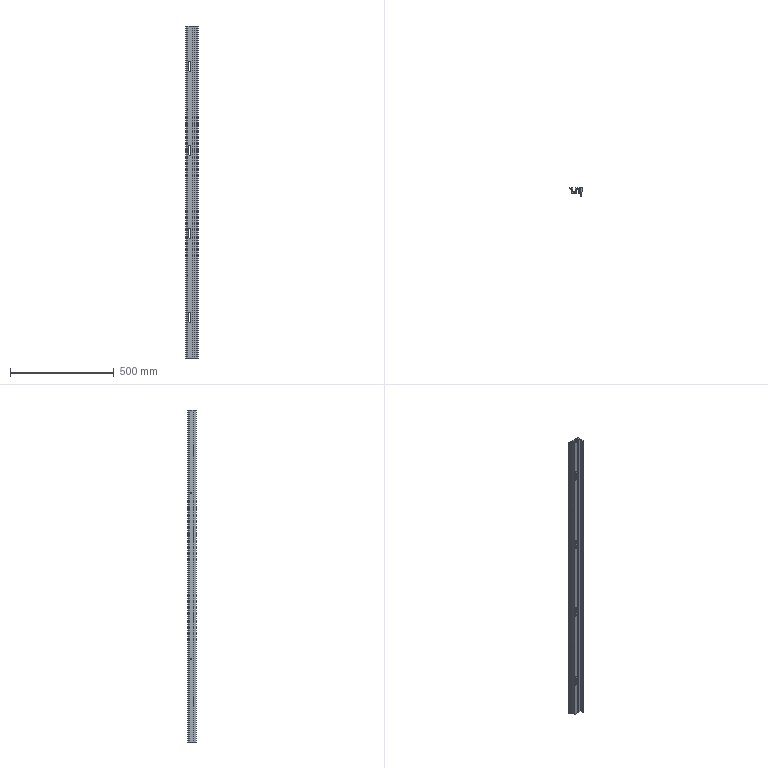Part | SolidWorks | features Emboss 1, Extrusion 1, ICE 1 | 1 solid | 74 faces | box 60 x 40 x 1600 mm | volume 1130094 mm3 | plane 50 | cylinder 24 | commonest cylinder face diameters 10 x12 2 x9 3 x2 4 x1